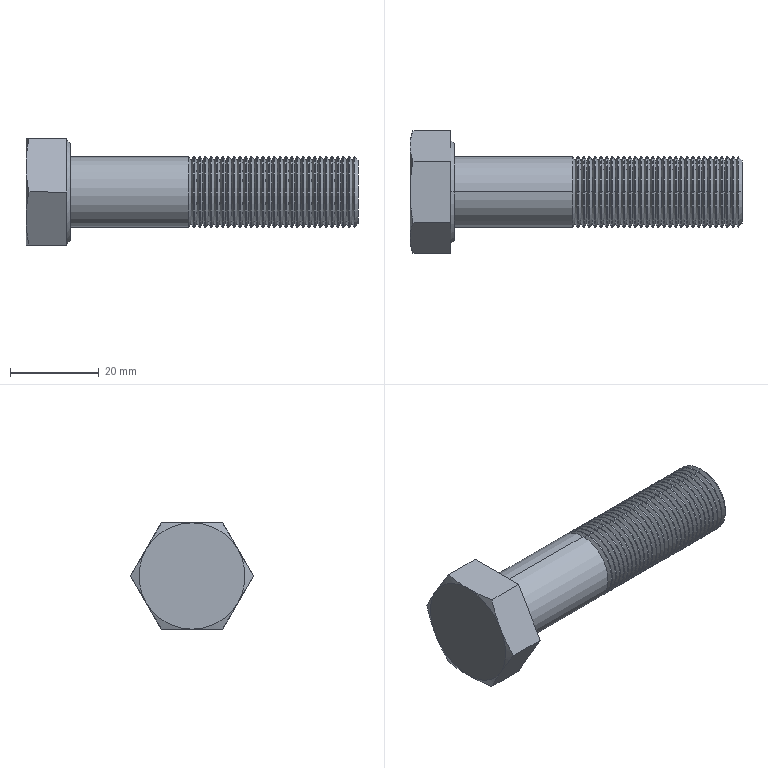Part | SolidWorks | features RevCut 3, Boss 1, Chamfer 1, Extrusion 1, Fillet 1, LPattern 1 | 1 solid | 194 faces | box 75 x 27.713 x 24 mm | volume 17249 mm3 | cone 126 | cylinder 58 | plane 10 | commonest cylinder face diameters 16 x58